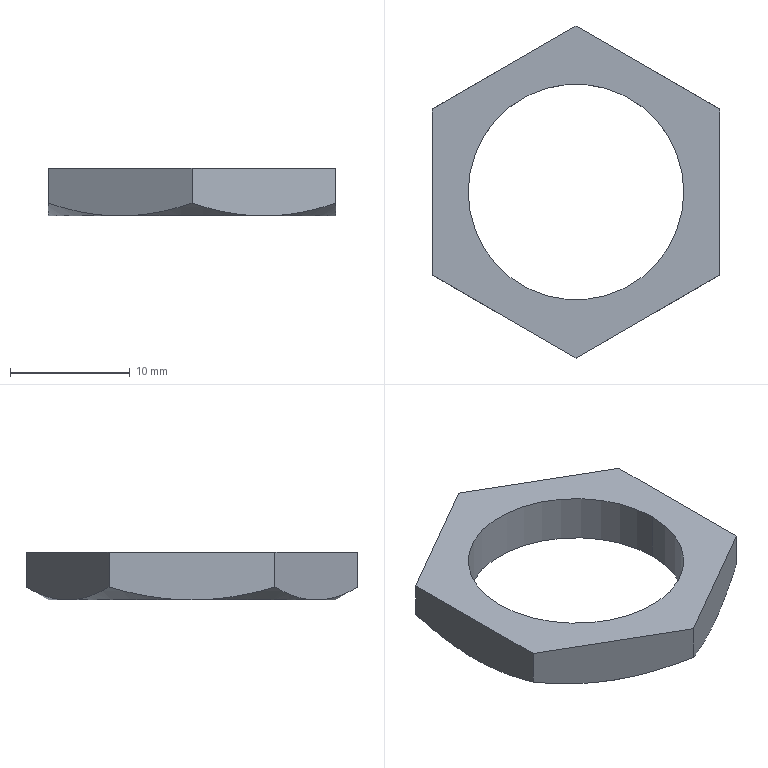Part | STEP file | E2EW-X7D118-M1TGJ0.3M-Part-2 | 1 solid | 16 faces | box 24 x 27.713 x 4 mm | volume 962.428 mm3 | plane 8 | cone 6 | cylinder 2 | commonest cylinder face diameters 18 x2